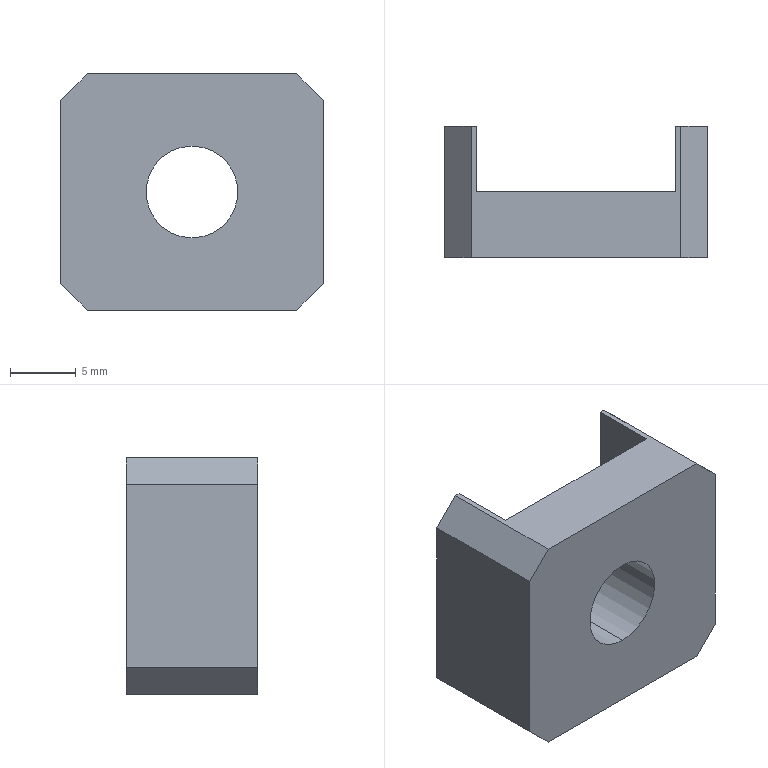Part | STEP file | con chan chot xien | 1 solid | 16 faces | box 20 x 10 x 18 mm | volume 1960 mm3 | plane 14 | cylinder 2 | commonest cylinder face diameters 7 x2
STEP:
#1=CARTESIAN_POINT('',(0.,0.,0.));
#2=DIRECTION('',(0.,0.,1.));
#3=DIRECTION('',(1.,0.,0.));
#4=AXIS2_PLACEMENT_3D('',#1,#2,#3);
#5=CARTESIAN_POINT('',(10.,5.,5.5));
#6=VERTEX_POINT('',#5);
#7=CARTESIAN_POINT('',(10.,0.,5.5));
#8=VERTEX_POINT('',#7);
#9=CARTESIAN_POINT('',(10.,28.705,5.5));
#10=DIRECTION('',(0.,-1.,0.));
#11=VECTOR('',#10,1.);
#12=LINE('',#9,#11);
#13=CARTESIAN_POINT('',(10.,28.705,9.));
#14=DIRECTION('',(0.,-1.,0.));
#15=DIRECTION('',(0.,0.,-1.));
#16=AXIS2_PLACEMENT_3D('',#13,#14,#15);
#17=CYLINDRICAL_SURFACE('',#16,3.5);
#18=CARTESIAN_POINT('',(6.283,0.));
#19=DIRECTION('',(0.,1.));
#20=VECTOR('',#19,1.);
#21=LINE('',#18,#20);
#22=(GEOMETRIC_REPRESENTATION_CONTEXT(2)PARAMETRIC_REPRESENTATION_CONTEXT()REPRESENTATION_CONTEXT('',''));
#23=DEFINITIONAL_REPRESENTATION('',(#21),#22);
#24=PCURVE('',#17,#23);
#25=CARTESIAN_POINT('',(10.,28.705,9.));
#26=DIRECTION('',(0.,-1.,0.));
#27=DIRECTION('',(0.,0.,-1.));
#28=AXIS2_PLACEMENT_3D('',#25,#26,#27);
#29=CYLINDRICAL_SURFACE('',#28,3.5);
#30=CARTESIAN_POINT('',(0.,0.));
#31=DIRECTION('',(0.,1.));
#32=VECTOR('',#31,1.);
#33=LINE('',#30,#32);
#34=(GEOMETRIC_REPRESENTATION_CONTEXT(2)PARAMETRIC_REPRESENTATION_CONTEXT()REPRESENTATION_CONTEXT('',''));
#35=DEFINITIONAL_REPRESENTATION('',(#33),#34);
#36=PCURVE('',#29,#35);
#37=SURFACE_CURVE('',#12,(#24,#36),.PCURVE_S1.);
#38=EDGE_CURVE('',#6,#8,#37,.T.);
#39=ORIENTED_EDGE('',*,*,#38,.T.);
#40=CARTESIAN_POINT('',(10.,0.,12.5));
#41=VERTEX_POINT('',#40);
#42=CARTESIAN_POINT('',(10.,0.,9.));
#43=DIRECTION('',(0.,1.,0.));
#44=DIRECTION('',(0.,0.,-1.));
#45=AXIS2_PLACEMENT_3D('',#42,#43,#44);
#46=CIRCLE('',#45,3.5);
#47=CARTESIAN_POINT('',(6.283,28.705));
#48=DIRECTION('',(-1.,0.));
#49=VECTOR('',#48,1.);
#50=LINE('',#47,#49);
#51=(GEOMETRIC_REPRESENTATION_CONTEXT(2)PARAMETRIC_REPRESENTATION_CONTEXT()REPRESENTATION_CONTEXT('',''));
#52=DEFINITIONAL_REPRESENTATION('',(#50),#51);
#53=PCURVE('',#17,#52);
#54=CARTESIAN_POINT('',(20.,0.,0.));
#55=DIRECTION('',(0.,-1.,0.));
#56=DIRECTION('',(0.,0.,-1.));
#57=AXIS2_PLACEMENT_3D('',#54,#55,#56);
#58=PLANE('',#57);
#59=CARTESIAN_POINT('',(-5.5,-10.));
#60=CARTESIAN_POINT('',(-5.5,-16.062));
#61=CARTESIAN_POINT('',(-10.75,-13.031));
#62=CARTESIAN_POINT('',(-16.,-10.));
#63=CARTESIAN_POINT('',(-10.75,-6.969));
#64=CARTESIAN_POINT('',(-5.5,-3.938));
#65=CARTESIAN_POINT('',(-5.5,-10.));
#66=(BOUNDED_CURVE()B_SPLINE_CURVE(2,(#59,#60,#61,#62,#63,#64,#65),.UNSPECIFIED.,.T.,.F.)B_SPLINE_CURVE_WITH_KNOTS((1,2,2,2,2,1),(-2.094,0.,2.094,4.189,6.283,8.378),.UNSPECIFIED.)CURVE()GEOMETRIC_REPRESENTATION_ITEM()RATIONAL_B_SPLINE_CURVE((1.,0.5,1.,0.5,1.,0.5,1.))REPRESENTATION_ITEM(''));
#67=(GEOMETRIC_REPRESENTATION_CONTEXT(2)PARAMETRIC_REPRESENTATION_CONTEXT()REPRESENTATION_CONTEXT('',''));
#68=DEFINITIONAL_REPRESENTATION('',(#66),#67);
#69=PCURVE('',#58,#68);
#70=SURFACE_CURVE('',#46,(#53,#69),.PCURVE_S1.);
#71=EDGE_CURVE('',#8,#41,#70,.T.);
#72=ORIENTED_EDGE('',*,*,#71,.T.);
#73=CARTESIAN_POINT('',(10.,5.,12.5));
#74=VERTEX_POINT('',#73);
#75=CARTESIAN_POINT('',(10.,28.705,12.5));
#76=DIRECTION('',(0.,-1.,0.));
#77=VECTOR('',#76,1.);
#78=LINE('',#75,#77);
#79=CARTESIAN_POINT('',(3.142,0.));
#80=DIRECTION('',(0.,1.));
#81=VECTOR('',#80,1.);
#82=LINE('',#79,#81);
#83=(GEOMETRIC_REPRESENTATION_CONTEXT(2)PARAMETRIC_REPRESENTATION_CONTEXT()REPRESENTATION_CONTEXT('',''));
#84=DEFINITIONAL_REPRESENTATION('',(#82),#83);
#85=PCURVE('',#17,#84);
#86=CARTESIAN_POINT('',(3.142,0.));
#87=DIRECTION('',(0.,1.));
#88=VECTOR('',#87,1.);
#89=LINE('',#86,#88);
#90=(GEOMETRIC_REPRESENTATION_CONTEXT(2)PARAMETRIC_REPRESENTATION_CONTEXT()REPRESENTATION_CONTEXT('',''));
#91=DEFINITIONAL_REPRESENTATION('',(#89),#90);
#92=PCURVE('',#29,#91);
#93=SURFACE_CURVE('',#78,(#85,#92),.PCURVE_S1.);
#94=EDGE_CURVE('',#74,#41,#93,.T.);
#95=ORIENTED_EDGE('',*,*,#94,.F.);
#96=CARTESIAN_POINT('',(10.,5.,9.));
#97=DIRECTION('',(0.,-1.,0.));
#98=DIRECTION('',(0.,0.,-1.));
#99=AXIS2_PLACEMENT_3D('',#96,#97,#98);
#100=CIRCLE('',#99,3.5);
#101=CARTESIAN_POINT('',(0.,23.705));
#102=DIRECTION('',(1.,0.));
#103=VECTOR('',#102,1.);
#104=LINE('',#101,#103);
#105=(GEOMETRIC_REPRESENTATION_CONTEXT(2)PARAMETRIC_REPRESENTATION_CONTEXT()REPRESENTATION_CONTEXT('',''));
#106=DEFINITIONAL_REPRESENTATION('',(#104),#105);
#107=PCURVE('',#17,#106);
#108=CARTESIAN_POINT('',(2.4,5.,0.));
#109=DIRECTION('',(0.,1.,0.));
#110=DIRECTION('',(0.,0.,1.));
#111=AXIS2_PLACEMENT_3D('',#108,#109,#110);
#112=PLANE('',#111);
#113=CARTESIAN_POINT('',(5.5,7.6));
#114=CARTESIAN_POINT('',(5.5,13.662));
#115=CARTESIAN_POINT('',(10.75,10.631));
#116=CARTESIAN_POINT('',(16.,7.6));
#117=CARTESIAN_POINT('',(10.75,4.569));
#118=CARTESIAN_POINT('',(5.5,1.538));
#119=CARTESIAN_POINT('',(5.5,7.6));
#120=(BOUNDED_CURVE()B_SPLINE_CURVE(2,(#113,#114,#115,#116,#117,#118,#119),.UNSPECIFIED.,.T.,.F.)B_SPLINE_CURVE_WITH_KNOTS((1,2,2,2,2,1),(-2.094,0.,2.094,4.189,6.283,8.378),.UNSPECIFIED.)CURVE()GEOMETRIC_REPRESENTATION_ITEM()RATIONAL_B_SPLINE_CURVE((1.,0.5,1.,0.5,1.,0.5,1.))REPRESENTATION_ITEM(''));
#121=(GEOMETRIC_REPRESENTATION_CONTEXT(2)PARAMETRIC_REPRESENTATION_CONTEXT()REPRESENTATION_CONTEXT('',''));
#122=DEFINITIONAL_REPRESENTATION('',(#120),#121);
#123=PCURVE('',#112,#122);
#124=SURFACE_CURVE('',#100,(#107,#123),.PCURVE_S1.);
#125=EDGE_CURVE('',#74,#6,#124,.T.);
#126=ORIENTED_EDGE('',*,*,#125,.T.);
#127=EDGE_LOOP('',(#39,#72,#95,#126));
#128=FACE_BOUND('',#127,.F.);
#129=ADVANCED_FACE('',(#128),#17,.F.);
#130=ORIENTED_EDGE('',*,*,#71,.T.);
#131=CARTESIAN_POINT('',(10.,0.,9.));
#132=DIRECTION('',(0.,1.,0.));
#133=DIRECTION('',(0.,0.,-1.));
#134=AXIS2_PLACEMENT_3D('',#131,#132,#133);
#135=CIRCLE('',#134,3.5);
#136=CARTESIAN_POINT('',(-5.5,-10.));
#137=CARTESIAN_POINT('',(-5.5,-16.062));
#138=CARTESIAN_POINT('',(-10.75,-13.031));
#139=CARTESIAN_POINT('',(-16.,-10.));
#140=CARTESIAN_POINT('',(-10.75,-6.969));
#141=CARTESIAN_POINT('',(-5.5,-3.938));
#142=CARTESIAN_POINT('',(-5.5,-10.));
#143=(BOUNDED_CURVE()B_SPLINE_CURVE(2,(#136,#137,#138,#139,#140,#141,#142),.UNSPECIFIED.,.T.,.F.)B_SPLINE_CURVE_WITH_KNOTS((1,2,2,2,2,1),(-2.094,0.,2.094,4.189,6.283,8.378),.UNSPECIFIED.)CURVE()GEOMETRIC_REPRESENTATION_ITEM()RATIONAL_B_SPLINE_CURVE((1.,0.5,1.,0.5,1.,0.5,1.))REPRESENTATION_ITEM(''));
#144=(GEOMETRIC_REPRESENTATION_CONTEXT(2)PARAMETRIC_REPRESENTATION_CONTEXT()REPRESENTATION_CONTEXT('',''));
#145=DEFINITIONAL_REPRESENTATION('',(#143),#144);
#146=PCURVE('',#58,#145);
#147=CARTESIAN_POINT('',(6.283,28.705));
#148=DIRECTION('',(-1.,0.));
#149=VECTOR('',#148,1.);
#150=LINE('',#147,#149);
#151=(GEOMETRIC_REPRESENTATION_CONTEXT(2)PARAMETRIC_REPRESENTATION_CONTEXT()REPRESENTATION_CONTEXT('',''));
#152=DEFINITIONAL_REPRESENTATION('',(#150),#151);
#153=PCURVE('',#29,#152);
#154=SURFACE_CURVE('',#135,(#146,#153),.PCURVE_S1.);
#155=EDGE_CURVE('',#41,#8,#154,.T.);
#156=ORIENTED_EDGE('',*,*,#155,.T.);
#157=EDGE_LOOP('',(#130,#156));
#158=FACE_BOUND('',#157,.T.);
#159=CARTESIAN_POINT('',(18.,0.,0.));
#160=VERTEX_POINT('',#159);
#161=CARTESIAN_POINT('',(20.,0.,2.));
#162=VERTEX_POINT('',#161);
#163=CARTESIAN_POINT('',(18.,0.,0.));
#164=DIRECTION('',(0.7071,0.,0.7071));
#165=VECTOR('',#164,1.);
#166=LINE('',#163,#165);
#167=CARTESIAN_POINT('',(0.,-2.));
#168=DIRECTION('',(-0.7071,0.7071));
#169=VECTOR('',#168,1.);
#170=LINE('',#167,#169);
#171=(GEOMETRIC_REPRESENTATION_CONTEXT(2)PARAMETRIC_REPRESENTATION_CONTEXT()REPRESENTATION_CONTEXT('',''));
#172=DEFINITIONAL_REPRESENTATION('',(#170),#171);
#173=PCURVE('',#58,#172);
#174=CARTESIAN_POINT('',(19.,7.136,1.));
#175=DIRECTION('',(0.7071,0.,-0.7071));
#176=DIRECTION('',(-0.7071,0.,-0.7071));
#177=AXIS2_PLACEMENT_3D('',#174,#175,#176);
#178=PLANE('',#177);
#179=CARTESIAN_POINT('',(1.414,-7.136));
#180=DIRECTION('',(-1.,0.));
#181=VECTOR('',#180,1.);
#182=LINE('',#179,#181);
#183=(GEOMETRIC_REPRESENTATION_CONTEXT(2)PARAMETRIC_REPRESENTATION_CONTEXT()REPRESENTATION_CONTEXT('',''));
#184=DEFINITIONAL_REPRESENTATION('',(#182),#183);
#185=PCURVE('',#178,#184);
#186=SURFACE_CURVE('',#166,(#173,#185),.PCURVE_S1.);
#187=EDGE_CURVE('',#160,#162,#186,.T.);
#188=ORIENTED_EDGE('',*,*,#187,.T.);
#189=CARTESIAN_POINT('',(20.,0.,16.));
#190=VERTEX_POINT('',#189);
#191=CARTESIAN_POINT('',(20.,0.,0.));
#192=DIRECTION('',(0.,0.,1.));
#193=VECTOR('',#192,1.);
#194=LINE('',#191,#193);
#195=CARTESIAN_POINT('',(0.,0.));
#196=DIRECTION('',(-1.,0.));
#197=VECTOR('',#196,1.);
#198=LINE('',#195,#197);
#199=(GEOMETRIC_REPRESENTATION_CONTEXT(2)PARAMETRIC_REPRESENTATION_CONTEXT()REPRESENTATION_CONTEXT('',''));
#200=DEFINITIONAL_REPRESENTATION('',(#198),#199);
#201=PCURVE('',#58,#200);
#202=CARTESIAN_POINT('',(20.,10.,0.));
#203=DIRECTION('',(1.,0.,0.));
#204=DIRECTION('',(0.,0.,-1.));
#205=AXIS2_PLACEMENT_3D('',#202,#203,#204);
#206=PLANE('',#205);
#207=CARTESIAN_POINT('',(0.,-10.));
#208=DIRECTION('',(-1.,0.));
#209=VECTOR('',#208,1.);
#210=LINE('',#207,#209);
#211=(GEOMETRIC_REPRESENTATION_CONTEXT(2)PARAMETRIC_REPRESENTATION_CONTEXT()REPRESENTATION_CONTEXT('',''));
#212=DEFINITIONAL_REPRESENTATION('',(#210),#211);
#213=PCURVE('',#206,#212);
#214=SURFACE_CURVE('',#194,(#201,#213),.PCURVE_S1.);
#215=EDGE_CURVE('',#162,#190,#214,.T.);
#216=ORIENTED_EDGE('',*,*,#215,.T.);
#217=CARTESIAN_POINT('',(18.,0.,18.));
#218=VERTEX_POINT('',#217);
#219=CARTESIAN_POINT('',(20.,0.,16.));
#220=DIRECTION('',(-0.7071,0.,0.7071));
#221=VECTOR('',#220,1.);
#222=LINE('',#219,#221);
#223=CARTESIAN_POINT('',(-16.,0.));
#224=DIRECTION('',(-0.7071,-0.7071));
#225=VECTOR('',#224,1.);
#226=LINE('',#223,#225);
#227=(GEOMETRIC_REPRESENTATION_CONTEXT(2)PARAMETRIC_REPRESENTATION_CONTEXT()REPRESENTATION_CONTEXT('',''));
#228=DEFINITIONAL_REPRESENTATION('',(#226),#227);
#229=PCURVE('',#58,#228);
#230=CARTESIAN_POINT('',(19.,7.136,17.));
#231=DIRECTION('',(0.7071,0.,0.7071));
#232=DIRECTION('',(0.7071,0.,-0.7071));
#233=AXIS2_PLACEMENT_3D('',#230,#231,#232);
#234=PLANE('',#233);
#235=CARTESIAN_POINT('',(1.414,-7.136));
#236=DIRECTION('',(-1.,0.));
#237=VECTOR('',#236,1.);
#238=LINE('',#235,#237);
#239=(GEOMETRIC_REPRESENTATION_CONTEXT(2)PARAMETRIC_REPRESENTATION_CONTEXT()REPRESENTATION_CONTEXT('',''));
#240=DEFINITIONAL_REPRESENTATION('',(#238),#239);
#241=PCURVE('',#234,#240);
#242=SURFACE_CURVE('',#222,(#229,#241),.PCURVE_S1.);
#243=EDGE_CURVE('',#190,#218,#242,.T.);
#244=ORIENTED_EDGE('',*,*,#243,.T.);
#245=CARTESIAN_POINT('',(2.,0.,18.));
#246=VERTEX_POINT('',#245);
#247=CARTESIAN_POINT('',(20.,0.,18.));
#248=DIRECTION('',(-1.,0.,0.));
#249=VECTOR('',#248,1.);
#250=LINE('',#247,#249);
#251=CARTESIAN_POINT('',(-18.,0.));
#252=DIRECTION('',(0.,-1.));
#253=VECTOR('',#252,1.);
#254=LINE('',#251,#253);
#255=(GEOMETRIC_REPRESENTATION_CONTEXT(2)PARAMETRIC_REPRESENTATION_CONTEXT()REPRESENTATION_CONTEXT('',''));
#256=DEFINITIONAL_REPRESENTATION('',(#254),#255);
#257=PCURVE('',#58,#256);
#258=CARTESIAN_POINT('',(10.,4.271,18.));
#259=DIRECTION('',(0.,0.,1.));
#260=DIRECTION('',(1.,0.,0.));
#261=AXIS2_PLACEMENT_3D('',#258,#259,#260);
#262=PLANE('',#261);
#263=CARTESIAN_POINT('',(10.,-4.271));
#264=DIRECTION('',(-1.,0.));
#265=VECTOR('',#264,1.);
#266=LINE('',#263,#265);
#267=(GEOMETRIC_REPRESENTATION_CONTEXT(2)PARAMETRIC_REPRESENTATION_CONTEXT()REPRESENTATION_CONTEXT('',''));
#268=DEFINITIONAL_REPRESENTATION('',(#266),#267);
#269=PCURVE('',#262,#268);
#270=SURFACE_CURVE('',#250,(#257,#269),.PCURVE_S1.);
#271=EDGE_CURVE('',#218,#246,#270,.T.);
#272=ORIENTED_EDGE('',*,*,#271,.T.);
#273=CARTESIAN_POINT('',(0.,0.,16.));
#274=VERTEX_POINT('',#273);
#275=CARTESIAN_POINT('',(2.,0.,18.));
#276=DIRECTION('',(-0.7071,0.,-0.7071));
#277=VECTOR('',#276,1.);
#278=LINE('',#275,#277);
#279=CARTESIAN_POINT('',(-18.,-18.));
#280=DIRECTION('',(0.7071,-0.7071));
#281=VECTOR('',#280,1.);
#282=LINE('',#279,#281);
#283=(GEOMETRIC_REPRESENTATION_CONTEXT(2)PARAMETRIC_REPRESENTATION_CONTEXT()REPRESENTATION_CONTEXT('',''));
#284=DEFINITIONAL_REPRESENTATION('',(#282),#283);
#285=PCURVE('',#58,#284);
#286=CARTESIAN_POINT('',(1.,2.136,17.));
#287=DIRECTION('',(-0.7071,0.,0.7071));
#288=DIRECTION('',(0.7071,0.,0.7071));
#289=AXIS2_PLACEMENT_3D('',#286,#287,#288);
#290=PLANE('',#289);
#291=CARTESIAN_POINT('',(1.414,-2.136));
#292=DIRECTION('',(-1.,0.));
#293=VECTOR('',#292,1.);
#294=LINE('',#291,#293);
#295=(GEOMETRIC_REPRESENTATION_CONTEXT(2)PARAMETRIC_REPRESENTATION_CONTEXT()REPRESENTATION_CONTEXT('',''));
#296=DEFINITIONAL_REPRESENTATION('',(#294),#295);
#297=PCURVE('',#290,#296);
#298=SURFACE_CURVE('',#278,(#285,#297),.PCURVE_S1.);
#299=EDGE_CURVE('',#246,#274,#298,.T.);
#300=ORIENTED_EDGE('',*,*,#299,.T.);
#301=CARTESIAN_POINT('',(0.,0.,2.));
#302=VERTEX_POINT('',#301);
#303=CARTESIAN_POINT('',(0.,0.,0.));
#304=DIRECTION('',(0.,0.,-1.));
#305=VECTOR('',#304,1.);
#306=LINE('',#303,#305);
#307=CARTESIAN_POINT('',(0.,-20.));
#308=DIRECTION('',(1.,0.));
#309=VECTOR('',#308,1.);
#310=LINE('',#307,#309);
#311=(GEOMETRIC_REPRESENTATION_CONTEXT(2)PARAMETRIC_REPRESENTATION_CONTEXT()REPRESENTATION_CONTEXT('',''));
#312=DEFINITIONAL_REPRESENTATION('',(#310),#311);
#313=PCURVE('',#58,#312);
#314=CARTESIAN_POINT('',(0.,0.,0.));
#315=DIRECTION('',(-1.,0.,0.));
#316=DIRECTION('',(0.,0.,1.));
#317=AXIS2_PLACEMENT_3D('',#314,#315,#316);
#318=PLANE('',#317);
#319=CARTESIAN_POINT('',(0.,0.));
#320=DIRECTION('',(-1.,0.));
#321=VECTOR('',#320,1.);
#322=LINE('',#319,#321);
#323=(GEOMETRIC_REPRESENTATION_CONTEXT(2)PARAMETRIC_REPRESENTATION_CONTEXT()REPRESENTATION_CONTEXT('',''));
#324=DEFINITIONAL_REPRESENTATION('',(#322),#323);
#325=PCURVE('',#318,#324);
#326=SURFACE_CURVE('',#306,(#313,#325),.PCURVE_S1.);
#327=EDGE_CURVE('',#274,#302,#326,.T.);
#328=ORIENTED_EDGE('',*,*,#327,.T.);
#329=CARTESIAN_POINT('',(2.,0.,0.));
#330=VERTEX_POINT('',#329);
#331=CARTESIAN_POINT('',(0.,0.,2.));
#332=DIRECTION('',(0.7071,0.,-0.7071));
#333=VECTOR('',#332,1.);
#334=LINE('',#331,#333);
#335=CARTESIAN_POINT('',(-2.,-20.));
#336=DIRECTION('',(0.7071,0.7071));
#337=VECTOR('',#336,1.);
#338=LINE('',#335,#337);
#339=(GEOMETRIC_REPRESENTATION_CONTEXT(2)PARAMETRIC_REPRESENTATION_CONTEXT()REPRESENTATION_CONTEXT('',''));
#340=DEFINITIONAL_REPRESENTATION('',(#338),#339);
#341=PCURVE('',#58,#340);
#342=CARTESIAN_POINT('',(1.,2.136,1.));
#343=DIRECTION('',(-0.7071,0.,-0.7071));
#344=DIRECTION('',(-0.7071,0.,0.7071));
#345=AXIS2_PLACEMENT_3D('',#342,#343,#344);
#346=PLANE('',#345);
#347=CARTESIAN_POINT('',(1.414,-2.136));
#348=DIRECTION('',(-1.,0.));
#349=VECTOR('',#348,1.);
#350=LINE('',#347,#349);
#351=(GEOMETRIC_REPRESENTATION_CONTEXT(2)PARAMETRIC_REPRESENTATION_CONTEXT()REPRESENTATION_CONTEXT('',''));
#352=DEFINITIONAL_REPRESENTATION('',(#350),#351);
#353=PCURVE('',#346,#352);
#354=SURFACE_CURVE('',#334,(#341,#353),.PCURVE_S1.);
#355=EDGE_CURVE('',#302,#330,#354,.T.);
#356=ORIENTED_EDGE('',*,*,#355,.T.);
#357=CARTESIAN_POINT('',(20.,0.,0.));
#358=DIRECTION('',(1.,0.,0.));
#359=VECTOR('',#358,1.);
#360=LINE('',#357,#359);
#361=CARTESIAN_POINT('',(0.,0.));
#362=DIRECTION('',(0.,1.));
#363=VECTOR('',#362,1.);
#364=LINE('',#361,#363);
#365=(GEOMETRIC_REPRESENTATION_CONTEXT(2)PARAMETRIC_REPRESENTATION_CONTEXT()REPRESENTATION_CONTEXT('',''));
#366=DEFINITIONAL_REPRESENTATION('',(#364),#365);
#367=PCURVE('',#58,#366);
#368=CARTESIAN_POINT('',(10.,4.271,0.));
#369=DIRECTION('',(0.,0.,1.));
#370=DIRECTION('',(1.,0.,0.));
#371=AXIS2_PLACEMENT_3D('',#368,#369,#370);
#372=PLANE('',#371);
#373=CARTESIAN_POINT('',(10.,-4.271));
#374=DIRECTION('',(1.,0.));
#375=VECTOR('',#374,1.);
#376=LINE('',#373,#375);
#377=(GEOMETRIC_REPRESENTATION_CONTEXT(2)PARAMETRIC_REPRESENTATION_CONTEXT()REPRESENTATION_CONTEXT('',''));
#378=DEFINITIONAL_REPRESENTATION('',(#376),#377);
#379=PCURVE('',#372,#378);
#380=SURFACE_CURVE('',#360,(#367,#379),.PCURVE_S1.);
#381=EDGE_CURVE('',#330,#160,#380,.T.);
#382=ORIENTED_EDGE('',*,*,#381,.T.);
#383=EDGE_LOOP('',(#188,#216,#244,#272,#300,#328,#356,#382));
#384=FACE_BOUND('',#383,.T.);
#385=ADVANCED_FACE('',(#158,#384),#58,.T.);
#386=ORIENTED_EDGE('',*,*,#155,.T.);
#387=ORIENTED_EDGE('',*,*,#38,.F.);
#388=CARTESIAN_POINT('',(10.,5.,9.));
#389=DIRECTION('',(0.,-1.,0.));
#390=DIRECTION('',(0.,0.,-1.));
#391=AXIS2_PLACEMENT_3D('',#388,#389,#390);
#392=CIRCLE('',#391,3.5);
#393=CARTESIAN_POINT('',(0.,23.705));
#394=DIRECTION('',(1.,0.));
#395=VECTOR('',#394,1.);
#396=LINE('',#393,#395);
#397=(GEOMETRIC_REPRESENTATION_CONTEXT(2)PARAMETRIC_REPRESENTATION_CONTEXT()REPRESENTATION_CONTEXT('',''));
#398=DEFINITIONAL_REPRESENTATION('',(#396),#397);
#399=PCURVE('',#29,#398);
#400=CARTESIAN_POINT('',(5.5,7.6));
#401=CARTESIAN_POINT('',(5.5,13.662));
#402=CARTESIAN_POINT('',(10.75,10.631));
#403=CARTESIAN_POINT('',(16.,7.6));
#404=CARTESIAN_POINT('',(10.75,4.569));
#405=CARTESIAN_POINT('',(5.5,1.538));
#406=CARTESIAN_POINT('',(5.5,7.6));
#407=(BOUNDED_CURVE()B_SPLINE_CURVE(2,(#400,#401,#402,#403,#404,#405,#406),.UNSPECIFIED.,.T.,.F.)B_SPLINE_CURVE_WITH_KNOTS((1,2,2,2,2,1),(-2.094,0.,2.094,4.189,6.283,8.378),.UNSPECIFIED.)CURVE()GEOMETRIC_REPRESENTATION_ITEM()RATIONAL_B_SPLINE_CURVE((1.,0.5,1.,0.5,1.,0.5,1.))REPRESENTATION_ITEM(''));
#408=(GEOMETRIC_REPRESENTATION_CONTEXT(2)PARAMETRIC_REPRESENTATION_CONTEXT()REPRESENTATION_CONTEXT('',''));
#409=DEFINITIONAL_REPRESENTATION('',(#407),#408);
#410=PCURVE('',#112,#409);
#411=SURFACE_CURVE('',#392,(#399,#410),.PCURVE_S1.);
#412=EDGE_CURVE('',#6,#74,#411,.T.);
#413=ORIENTED_EDGE('',*,*,#412,.T.);
#414=ORIENTED_EDGE('',*,*,#94,.T.);
#415=EDGE_LOOP('',(#386,#387,#413,#414));
#416=FACE_BOUND('',#415,.F.);
#417=ADVANCED_FACE('',(#416),#29,.F.);
#418=CARTESIAN_POINT('',(20.,10.,2.));
#419=VERTEX_POINT('',#418);
#420=CARTESIAN_POINT('',(20.,10.,2.));
#421=DIRECTION('',(0.,1.,0.));
#422=VECTOR('',#421,1.);
#423=LINE('',#420,#422);
#424=CARTESIAN_POINT('',(-2.,0.));
#425=DIRECTION('',(0.,1.));
#426=VECTOR('',#425,1.);
#427=LINE('',#424,#426);
#428=(GEOMETRIC_REPRESENTATION_CONTEXT(2)PARAMETRIC_REPRESENTATION_CONTEXT()REPRESENTATION_CONTEXT('',''));
#429=DEFINITIONAL_REPRESENTATION('',(#427),#428);
#430=PCURVE('',#206,#429);
#431=CARTESIAN_POINT('',(-1.414,2.864));
#432=DIRECTION('',(0.,1.));
#433=VECTOR('',#432,1.);
#434=LINE('',#431,#433);
#435=(GEOMETRIC_REPRESENTATION_CONTEXT(2)PARAMETRIC_REPRESENTATION_CONTEXT()REPRESENTATION_CONTEXT('',''));
#436=DEFINITIONAL_REPRESENTATION('',(#434),#435);
#437=PCURVE('',#178,#436);
#438=SURFACE_CURVE('',#423,(#430,#437),.PCURVE_S1.);
#439=EDGE_CURVE('',#162,#419,#438,.T.);
#440=ORIENTED_EDGE('',*,*,#439,.T.);
#441=CARTESIAN_POINT('',(20.,10.,16.));
#442=VERTEX_POINT('',#441);
#443=CARTESIAN_POINT('',(20.,10.,0.));
#444=DIRECTION('',(0.,0.,1.));
#445=VECTOR('',#444,1.);
#446=LINE('',#443,#445);
#447=CARTESIAN_POINT('',(0.,0.));
#448=DIRECTION('',(-1.,0.));
#449=VECTOR('',#448,1.);
#450=LINE('',#447,#449);
#451=(GEOMETRIC_REPRESENTATION_CONTEXT(2)PARAMETRIC_REPRESENTATION_CONTEXT()REPRESENTATION_CONTEXT('',''));
#452=DEFINITIONAL_REPRESENTATION('',(#450),#451);
#453=PCURVE('',#206,#452);
#454=CARTESIAN_POINT('',(17.6,10.,0.));
#455=DIRECTION('',(0.,1.,0.));
#456=DIRECTION('',(0.,0.,1.));
#457=AXIS2_PLACEMENT_3D('',#454,#455,#456);
#458=PLANE('',#457);
#459=CARTESIAN_POINT('',(0.,2.4));
#460=DIRECTION('',(1.,0.));
#461=VECTOR('',#460,1.);
#462=LINE('',#459,#461);
#463=(GEOMETRIC_REPRESENTATION_CONTEXT(2)PARAMETRIC_REPRESENTATION_CONTEXT()REPRESENTATION_CONTEXT('',''));
#464=DEFINITIONAL_REPRESENTATION('',(#462),#463);
#465=PCURVE('',#458,#464);
#466=SURFACE_CURVE('',#446,(#453,#465),.PCURVE_S1.);
#467=EDGE_CURVE('',#419,#442,#466,.T.);
#468=ORIENTED_EDGE('',*,*,#467,.T.);
#469=CARTESIAN_POINT('',(20.,10.,16.));
#470=DIRECTION('',(0.,-1.,0.));
#471=VECTOR('',#470,1.);
#472=LINE('',#469,#471);
#473=CARTESIAN_POINT('',(-16.,0.));
#474=DIRECTION('',(0.,-1.));
#475=VECTOR('',#474,1.);
#476=LINE('',#473,#475);
#477=(GEOMETRIC_REPRESENTATION_CONTEXT(2)PARAMETRIC_REPRESENTATION_CONTEXT()REPRESENTATION_CONTEXT('',''));
#478=DEFINITIONAL_REPRESENTATION('',(#476),#477);
#479=PCURVE('',#206,#478);
#480=CARTESIAN_POINT('',(1.414,2.864));
#481=DIRECTION('',(0.,-1.));
#482=VECTOR('',#481,1.);
#483=LINE('',#480,#482);
#484=(GEOMETRIC_REPRESENTATION_CONTEXT(2)PARAMETRIC_REPRESENTATION_CONTEXT()REPRESENTATION_CONTEXT('',''));
#485=DEFINITIONAL_REPRESENTATION('',(#483),#484);
#486=PCURVE('',#234,#485);
#487=SURFACE_CURVE('',#472,(#479,#486),.PCURVE_S1.);
#488=EDGE_CURVE('',#442,#190,#487,.T.);
#489=ORIENTED_EDGE('',*,*,#488,.T.);
#490=ORIENTED_EDGE('',*,*,#215,.F.);
#491=EDGE_LOOP('',(#440,#468,#489,#490));
#492=FACE_BOUND('',#491,.T.);
#493=ADVANCED_FACE('',(#492),#206,.T.);
#494=ORIENTED_EDGE('',*,*,#187,.F.);
#495=CARTESIAN_POINT('',(18.,10.,0.));
#496=VERTEX_POINT('',#495);
#497=CARTESIAN_POINT('',(18.,7.136,0.));
#498=DIRECTION('',(0.,1.,0.));
#499=VECTOR('',#498,1.);
#500=LINE('',#497,#499);
#501=CARTESIAN_POINT('',(1.414,0.));
#502=DIRECTION('',(0.,1.));
#503=VECTOR('',#502,1.);
#504=LINE('',#501,#503);
#505=(GEOMETRIC_REPRESENTATION_CONTEXT(2)PARAMETRIC_REPRESENTATION_CONTEXT()REPRESENTATION_CONTEXT('',''));
#506=DEFINITIONAL_REPRESENTATION('',(#504),#505);
#507=PCURVE('',#178,#506);
#508=CARTESIAN_POINT('',(8.,2.864));
#509=DIRECTION('',(0.,1.));
#510=VECTOR('',#509,1.);
#511=LINE('',#508,#510);
#512=(GEOMETRIC_REPRESENTATION_CONTEXT(2)PARAMETRIC_REPRESENTATION_CONTEXT()REPRESENTATION_CONTEXT('',''));
#513=DEFINITIONAL_REPRESENTATION('',(#511),#512);
#514=PCURVE('',#372,#513);
#515=SURFACE_CURVE('',#500,(#507,#514),.PCURVE_S1.);
#516=EDGE_CURVE('',#160,#496,#515,.T.);
#517=ORIENTED_EDGE('',*,*,#516,.T.);
#518=CARTESIAN_POINT('',(19.,10.,1.));
#519=DIRECTION('',(0.7071,0.,0.7071));
#520=VECTOR('',#519,1.);
#521=LINE('',#518,#520);
#522=CARTESIAN_POINT('',(0.,2.864));
#523=DIRECTION('',(-1.,0.));
#524=VECTOR('',#523,1.);
#525=LINE('',#522,#524);
#526=(GEOMETRIC_REPRESENTATION_CONTEXT(2)PARAMETRIC_REPRESENTATION_CONTEXT()REPRESENTATION_CONTEXT('',''));
#527=DEFINITIONAL_REPRESENTATION('',(#525),#526);
#528=PCURVE('',#178,#527);
#529=CARTESIAN_POINT('',(1.,1.4));
#530=DIRECTION('',(0.7071,0.7071));
#531=VECTOR('',#530,1.);
#532=LINE('',#529,#531);
#533=(GEOMETRIC_REPRESENTATION_CONTEXT(2)PARAMETRIC_REPRESENTATION_CONTEXT()REPRESENTATION_CONTEXT('',''));
#534=DEFINITIONAL_REPRESENTATION('',(#532),#533);
#535=PCURVE('',#458,#534);
#536=SURFACE_CURVE('',#521,(#528,#535),.PCURVE_S1.);
#537=EDGE_CURVE('',#496,#419,#536,.T.);
#538=ORIENTED_EDGE('',*,*,#537,.T.);
#539=ORIENTED_EDGE('',*,*,#439,.F.);
#540=EDGE_LOOP('',(#494,#517,#538,#539));
#541=FACE_BOUND('',#540,.T.);
#542=ADVANCED_FACE('',(#541),#178,.T.);
#543=ORIENTED_EDGE('',*,*,#381,.F.);
#544=CARTESIAN_POINT('',(2.,10.,0.));
#545=VERTEX_POINT('',#544);
#546=CARTESIAN_POINT('',(2.,4.271,0.));
#547=DIRECTION('',(0.,-1.,0.));
#548=VECTOR('',#547,1.);
#549=LINE('',#546,#548);
#550=CARTESIAN_POINT('',(-8.,0.));
#551=DIRECTION('',(0.,-1.));
#552=VECTOR('',#551,1.);
#553=LINE('',#550,#552);
#554=(GEOMETRIC_REPRESENTATION_CONTEXT(2)PARAMETRIC_REPRESENTATION_CONTEXT()REPRESENTATION_CONTEXT('',''));
#555=DEFINITIONAL_REPRESENTATION('',(#553),#554);
#556=PCURVE('',#372,#555);
#557=CARTESIAN_POINT('',(-1.414,2.136));
#558=DIRECTION('',(0.,-1.));
#559=VECTOR('',#558,1.);
#560=LINE('',#557,#559);
#561=(GEOMETRIC_REPRESENTATION_CONTEXT(2)PARAMETRIC_REPRESENTATION_CONTEXT()REPRESENTATION_CONTEXT('',''));
#562=DEFINITIONAL_REPRESENTATION('',(#560),#561);
#563=PCURVE('',#346,#562);
#564=SURFACE_CURVE('',#549,(#556,#563),.PCURVE_S1.);
#565=EDGE_CURVE('',#545,#330,#564,.T.);
#566=ORIENTED_EDGE('',*,*,#565,.F.);
#567=CARTESIAN_POINT('',(2.4,10.,0.));
#568=VERTEX_POINT('',#567);
#569=CARTESIAN_POINT('',(0.,10.,0.));
#570=DIRECTION('',(-1.,0.,0.));
#571=VECTOR('',#570,1.);
#572=LINE('',#569,#571);
#573=CARTESIAN_POINT('',(-10.,5.729));
#574=DIRECTION('',(-1.,0.));
#575=VECTOR('',#574,1.);
#576=LINE('',#573,#575);
#577=(GEOMETRIC_REPRESENTATION_CONTEXT(2)PARAMETRIC_REPRESENTATION_CONTEXT()REPRESENTATION_CONTEXT('',''));
#578=DEFINITIONAL_REPRESENTATION('',(#576),#577);
#579=PCURVE('',#372,#578);
#580=CARTESIAN_POINT('',(0.,10.,0.));
#581=DIRECTION('',(0.,1.,0.));
#582=DIRECTION('',(0.,0.,1.));
#583=AXIS2_PLACEMENT_3D('',#580,#581,#582);
#584=PLANE('',#583);
#585=CARTESIAN_POINT('',(0.,0.));
#586=DIRECTION('',(0.,-1.));
#587=VECTOR('',#586,1.);
#588=LINE('',#585,#587);
#589=(GEOMETRIC_REPRESENTATION_CONTEXT(2)PARAMETRIC_REPRESENTATION_CONTEXT()REPRESENTATION_CONTEXT('',''));
#590=DEFINITIONAL_REPRESENTATION('',(#588),#589);
#591=PCURVE('',#584,#590);
#592=SURFACE_CURVE('',#572,(#579,#591),.PCURVE_S1.);
#593=EDGE_CURVE('',#568,#545,#592,.T.);
#594=ORIENTED_EDGE('',*,*,#593,.F.);
#595=CARTESIAN_POINT('',(2.4,5.,0.));
#596=VERTEX_POINT('',#595);
#597=CARTESIAN_POINT('',(2.4,4.271,0.));
#598=DIRECTION('',(0.,1.,0.));
#599=VECTOR('',#598,1.);
#600=LINE('',#597,#599);
#601=CARTESIAN_POINT('',(-7.6,0.));
#602=DIRECTION('',(0.,1.));
#603=VECTOR('',#602,1.);
#604=LINE('',#601,#603);
#605=(GEOMETRIC_REPRESENTATION_CONTEXT(2)PARAMETRIC_REPRESENTATION_CONTEXT()REPRESENTATION_CONTEXT('',''));
#606=DEFINITIONAL_REPRESENTATION('',(#604),#605);
#607=PCURVE('',#372,#606);
#608=CARTESIAN_POINT('',(2.4,10.,0.));
#609=DIRECTION('',(1.,0.,0.));
#610=DIRECTION('',(0.,0.,-1.));
#611=AXIS2_PLACEMENT_3D('',#608,#609,#610);
#612=PLANE('',#611);
#613=CARTESIAN_POINT('',(0.,-5.729));
#614=DIRECTION('',(0.,1.));
#615=VECTOR('',#614,1.);
#616=LINE('',#613,#615);
#617=(GEOMETRIC_REPRESENTATION_CONTEXT(2)PARAMETRIC_REPRESENTATION_CONTEXT()REPRESENTATION_CONTEXT('',''));
#618=DEFINITIONAL_REPRESENTATION('',(#616),#617);
#619=PCURVE('',#612,#618);
#620=SURFACE_CURVE('',#600,(#607,#619),.PCURVE_S1.);
#621=EDGE_CURVE('',#596,#568,#620,.T.);
#622=ORIENTED_EDGE('',*,*,#621,.F.);
#623=CARTESIAN_POINT('',(17.6,5.,0.));
#624=VERTEX_POINT('',#623);
#625=CARTESIAN_POINT('',(10.,5.,0.));
#626=DIRECTION('',(-1.,0.,0.));
#627=VECTOR('',#626,1.);
#628=LINE('',#625,#627);
#629=CARTESIAN_POINT('',(0.,0.7286));
#630=DIRECTION('',(-1.,0.));
#631=VECTOR('',#630,1.);
#632=LINE('',#629,#631);
#633=(GEOMETRIC_REPRESENTATION_CONTEXT(2)PARAMETRIC_REPRESENTATION_CONTEXT()REPRESENTATION_CONTEXT('',''));
#634=DEFINITIONAL_REPRESENTATION('',(#632),#633);
#635=PCURVE('',#372,#634);
#636=CARTESIAN_POINT('',(0.,7.6));
#637=DIRECTION('',(0.,-1.));
#638=VECTOR('',#637,1.);
#639=LINE('',#636,#638);
#640=(GEOMETRIC_REPRESENTATION_CONTEXT(2)PARAMETRIC_REPRESENTATION_CONTEXT()REPRESENTATION_CONTEXT('',''));
#641=DEFINITIONAL_REPRESENTATION('',(#639),#640);
#642=PCURVE('',#112,#641);
#643=SURFACE_CURVE('',#628,(#635,#642),.PCURVE_S1.);
#644=EDGE_CURVE('',#624,#596,#643,.T.);
#645=ORIENTED_EDGE('',*,*,#644,.F.);
#646=CARTESIAN_POINT('',(17.6,10.,0.));
#647=VERTEX_POINT('',#646);
#648=CARTESIAN_POINT('',(17.6,4.271,0.));
#649=DIRECTION('',(0.,-1.,0.));
#650=VECTOR('',#649,1.);
#651=LINE('',#648,#650);
#652=CARTESIAN_POINT('',(7.6,0.));
#653=DIRECTION('',(0.,-1.));
#654=VECTOR('',#653,1.);
#655=LINE('',#652,#654);
#656=(GEOMETRIC_REPRESENTATION_CONTEXT(2)PARAMETRIC_REPRESENTATION_CONTEXT()REPRESENTATION_CONTEXT('',''));
#657=DEFINITIONAL_REPRESENTATION('',(#655),#656);
#658=PCURVE('',#372,#657);
#659=CARTESIAN_POINT('',(17.6,5.,0.));
#660=DIRECTION('',(-1.,0.,0.));
#661=DIRECTION('',(0.,0.,1.));
#662=AXIS2_PLACEMENT_3D('',#659,#660,#661);
#663=PLANE('',#662);
#664=CARTESIAN_POINT('',(0.,-0.7286));
#665=DIRECTION('',(0.,-1.));
#666=VECTOR('',#665,1.);
#667=LINE('',#664,#666);
#668=(GEOMETRIC_REPRESENTATION_CONTEXT(2)PARAMETRIC_REPRESENTATION_CONTEXT()REPRESENTATION_CONTEXT('',''));
#669=DEFINITIONAL_REPRESENTATION('',(#667),#668);
#670=PCURVE('',#663,#669);
#671=SURFACE_CURVE('',#651,(#658,#670),.PCURVE_S1.);
#672=EDGE_CURVE('',#647,#624,#671,.T.);
#673=ORIENTED_EDGE('',*,*,#672,.F.);
#674=CARTESIAN_POINT('',(10.,10.,0.));
#675=DIRECTION('',(-1.,0.,0.));
#676=VECTOR('',#675,1.);
#677=LINE('',#674,#676);
#678=CARTESIAN_POINT('',(0.,5.729));
#679=DIRECTION('',(-1.,0.));
#680=VECTOR('',#679,1.);
#681=LINE('',#678,#680);
#682=(GEOMETRIC_REPRESENTATION_CONTEXT(2)PARAMETRIC_REPRESENTATION_CONTEXT()REPRESENTATION_CONTEXT('',''));
#683=DEFINITIONAL_REPRESENTATION('',(#681),#682);
#684=PCURVE('',#372,#683);
#685=CARTESIAN_POINT('',(0.,-7.6));
#686=DIRECTION('',(0.,-1.));
#687=VECTOR('',#686,1.);
#688=LINE('',#685,#687);
#689=(GEOMETRIC_REPRESENTATION_CONTEXT(2)PARAMETRIC_REPRESENTATION_CONTEXT()REPRESENTATION_CONTEXT('',''));
#690=DEFINITIONAL_REPRESENTATION('',(#688),#689);
#691=PCURVE('',#458,#690);
#692=SURFACE_CURVE('',#677,(#684,#691),.PCURVE_S1.);
#693=EDGE_CURVE('',#496,#647,#692,.T.);
#694=ORIENTED_EDGE('',*,*,#693,.F.);
#695=ORIENTED_EDGE('',*,*,#516,.F.);
#696=EDGE_LOOP('',(#543,#566,#594,#622,#645,#673,#694,#695));
#697=FACE_BOUND('',#696,.T.);
#698=ADVANCED_FACE('',(#697),#372,.F.);
#699=CARTESIAN_POINT('',(0.,10.,2.));
#700=VERTEX_POINT('',#699);
#701=CARTESIAN_POINT('',(1.,10.,1.));
#702=DIRECTION('',(0.7071,0.,-0.7071));
#703=VECTOR('',#702,1.);
#704=LINE('',#701,#703);
#705=CARTESIAN_POINT('',(0.,7.864));
#706=DIRECTION('',(-1.,0.));
#707=VECTOR('',#706,1.);
#708=LINE('',#705,#707);
#709=(GEOMETRIC_REPRESENTATION_CONTEXT(2)PARAMETRIC_REPRESENTATION_CONTEXT()REPRESENTATION_CONTEXT('',''));
#710=DEFINITIONAL_REPRESENTATION('',(#708),#709);
#711=PCURVE('',#346,#710);
#712=CARTESIAN_POINT('',(1.,1.));
#713=DIRECTION('',(-0.7071,0.7071));
#714=VECTOR('',#713,1.);
#715=LINE('',#712,#714);
#716=(GEOMETRIC_REPRESENTATION_CONTEXT(2)PARAMETRIC_REPRESENTATION_CONTEXT()REPRESENTATION_CONTEXT('',''));
#717=DEFINITIONAL_REPRESENTATION('',(#715),#716);
#718=PCURVE('',#584,#717);
#719=SURFACE_CURVE('',#704,(#711,#718),.PCURVE_S1.);
#720=EDGE_CURVE('',#700,#545,#719,.T.);
#721=ORIENTED_EDGE('',*,*,#720,.T.);
#722=ORIENTED_EDGE('',*,*,#565,.T.);
#723=ORIENTED_EDGE('',*,*,#355,.F.);
#724=CARTESIAN_POINT('',(0.,2.136,2.));
#725=DIRECTION('',(0.,1.,0.));
#726=VECTOR('',#725,1.);
#727=LINE('',#724,#726);
#728=CARTESIAN_POINT('',(1.414,0.));
#729=DIRECTION('',(0.,1.));
#730=VECTOR('',#729,1.);
#731=LINE('',#728,#730);
#732=(GEOMETRIC_REPRESENTATION_CONTEXT(2)PARAMETRIC_REPRESENTATION_CONTEXT()REPRESENTATION_CONTEXT('',''));
#733=DEFINITIONAL_REPRESENTATION('',(#731),#732);
#734=PCURVE('',#346,#733);
#735=CARTESIAN_POINT('',(2.,2.136));
#736=DIRECTION('',(0.,1.));
#737=VECTOR('',#736,1.);
#738=LINE('',#735,#737);
#739=(GEOMETRIC_REPRESENTATION_CONTEXT(2)PARAMETRIC_REPRESENTATION_CONTEXT()REPRESENTATION_CONTEXT('',''));
#740=DEFINITIONAL_REPRESENTATION('',(#738),#739);
#741=PCURVE('',#318,#740);
#742=SURFACE_CURVE('',#727,(#734,#741),.PCURVE_S1.);
#743=EDGE_CURVE('',#302,#700,#742,.T.);
#744=ORIENTED_EDGE('',*,*,#743,.T.);
#745=EDGE_LOOP('',(#721,#722,#723,#744));
#746=FACE_BOUND('',#745,.T.);
#747=ADVANCED_FACE('',(#746),#346,.T.);
#748=CARTESIAN_POINT('',(0.,10.,16.));
#749=VERTEX_POINT('',#748);
#750=CARTESIAN_POINT('',(0.,0.,16.));
#751=DIRECTION('',(0.,1.,0.));
#752=VECTOR('',#751,1.);
#753=LINE('',#750,#752);
#754=CARTESIAN_POINT('',(16.,0.));
#755=DIRECTION('',(0.,1.));
#756=VECTOR('',#755,1.);
#757=LINE('',#754,#756);
#758=(GEOMETRIC_REPRESENTATION_CONTEXT(2)PARAMETRIC_REPRESENTATION_CONTEXT()REPRESENTATION_CONTEXT('',''));
#759=DEFINITIONAL_REPRESENTATION('',(#757),#758);
#760=PCURVE('',#318,#759);
#761=CARTESIAN_POINT('',(-1.414,-2.136));
#762=DIRECTION('',(0.,1.));
#763=VECTOR('',#762,1.);
#764=LINE('',#761,#763);
#765=(GEOMETRIC_REPRESENTATION_CONTEXT(2)PARAMETRIC_REPRESENTATION_CONTEXT()REPRESENTATION_CONTEXT('',''));
#766=DEFINITIONAL_REPRESENTATION('',(#764),#765);
#767=PCURVE('',#290,#766);
#768=SURFACE_CURVE('',#753,(#760,#767),.PCURVE_S1.);
#769=EDGE_CURVE('',#274,#749,#768,.T.);
#770=ORIENTED_EDGE('',*,*,#769,.T.);
#771=CARTESIAN_POINT('',(0.,10.,0.));
#772=DIRECTION('',(0.,0.,-1.));
#773=VECTOR('',#772,1.);
#774=LINE('',#771,#773);
#775=CARTESIAN_POINT('',(0.,10.));
#776=DIRECTION('',(-1.,0.));
#777=VECTOR('',#776,1.);
#778=LINE('',#775,#777);
#779=(GEOMETRIC_REPRESENTATION_CONTEXT(2)PARAMETRIC_REPRESENTATION_CONTEXT()REPRESENTATION_CONTEXT('',''));
#780=DEFINITIONAL_REPRESENTATION('',(#778),#779);
#781=PCURVE('',#318,#780);
#782=CARTESIAN_POINT('',(0.,0.));
#783=DIRECTION('',(-1.,0.));
#784=VECTOR('',#783,1.);
#785=LINE('',#782,#784);
#786=(GEOMETRIC_REPRESENTATION_CONTEXT(2)PARAMETRIC_REPRESENTATION_CONTEXT()REPRESENTATION_CONTEXT('',''));
#787=DEFINITIONAL_REPRESENTATION('',(#785),#786);
#788=PCURVE('',#584,#787);
#789=SURFACE_CURVE('',#774,(#781,#788),.PCURVE_S1.);
#790=EDGE_CURVE('',#749,#700,#789,.T.);
#791=ORIENTED_EDGE('',*,*,#790,.T.);
#792=ORIENTED_EDGE('',*,*,#743,.F.);
#793=ORIENTED_EDGE('',*,*,#327,.F.);
#794=EDGE_LOOP('',(#770,#791,#792,#793));
#795=FACE_BOUND('',#794,.T.);
#796=ADVANCED_FACE('',(#795),#318,.T.);
#797=ORIENTED_EDGE('',*,*,#299,.F.);
#798=CARTESIAN_POINT('',(2.,10.,18.));
#799=VERTEX_POINT('',#798);
#800=CARTESIAN_POINT('',(2.,2.136,18.));
#801=DIRECTION('',(0.,1.,0.));
#802=VECTOR('',#801,1.);
#803=LINE('',#800,#802);
#804=CARTESIAN_POINT('',(1.414,0.));
#805=DIRECTION('',(0.,1.));
#806=VECTOR('',#805,1.);
#807=LINE('',#804,#806);
#808=(GEOMETRIC_REPRESENTATION_CONTEXT(2)PARAMETRIC_REPRESENTATION_CONTEXT()REPRESENTATION_CONTEXT('',''));
#809=DEFINITIONAL_REPRESENTATION('',(#807),#808);
#810=PCURVE('',#290,#809);
#811=CARTESIAN_POINT('',(-8.,-2.136));
#812=DIRECTION('',(0.,1.));
#813=VECTOR('',#812,1.);
#814=LINE('',#811,#813);
#815=(GEOMETRIC_REPRESENTATION_CONTEXT(2)PARAMETRIC_REPRESENTATION_CONTEXT()REPRESENTATION_CONTEXT('',''));
#816=DEFINITIONAL_REPRESENTATION('',(#814),#815);
#817=PCURVE('',#262,#816);
#818=SURFACE_CURVE('',#803,(#810,#817),.PCURVE_S1.);
#819=EDGE_CURVE('',#246,#799,#818,.T.);
#820=ORIENTED_EDGE('',*,*,#819,.T.);
#821=CARTESIAN_POINT('',(1.,10.,17.));
#822=DIRECTION('',(-0.7071,0.,-0.7071));
#823=VECTOR('',#822,1.);
#824=LINE('',#821,#823);
#825=CARTESIAN_POINT('',(0.,7.864));
#826=DIRECTION('',(-1.,0.));
#827=VECTOR('',#826,1.);
#828=LINE('',#825,#827);
#829=(GEOMETRIC_REPRESENTATION_CONTEXT(2)PARAMETRIC_REPRESENTATION_CONTEXT()REPRESENTATION_CONTEXT('',''));
#830=DEFINITIONAL_REPRESENTATION('',(#828),#829);
#831=PCURVE('',#290,#830);
#832=CARTESIAN_POINT('',(17.,1.));
#833=DIRECTION('',(-0.7071,-0.7071));
#834=VECTOR('',#833,1.);
#835=LINE('',#832,#834);
#836=(GEOMETRIC_REPRESENTATION_CONTEXT(2)PARAMETRIC_REPRESENTATION_CONTEXT()REPRESENTATION_CONTEXT('',''));
#837=DEFINITIONAL_REPRESENTATION('',(#835),#836);
#838=PCURVE('',#584,#837);
#839=SURFACE_CURVE('',#824,(#831,#838),.PCURVE_S1.);
#840=EDGE_CURVE('',#799,#749,#839,.T.);
#841=ORIENTED_EDGE('',*,*,#840,.T.);
#842=ORIENTED_EDGE('',*,*,#769,.F.);
#843=EDGE_LOOP('',(#797,#820,#841,#842));
#844=FACE_BOUND('',#843,.T.);
#845=ADVANCED_FACE('',(#844),#290,.T.);
#846=ORIENTED_EDGE('',*,*,#819,.F.);
#847=ORIENTED_EDGE('',*,*,#271,.F.);
#848=CARTESIAN_POINT('',(18.,10.,18.));
#849=VERTEX_POINT('',#848);
#850=CARTESIAN_POINT('',(18.,4.271,18.));
#851=DIRECTION('',(0.,1.,0.));
#852=VECTOR('',#851,1.);
#853=LINE('',#850,#852);
#854=CARTESIAN_POINT('',(8.,0.));
#855=DIRECTION('',(0.,1.));
#856=VECTOR('',#855,1.);
#857=LINE('',#854,#856);
#858=(GEOMETRIC_REPRESENTATION_CONTEXT(2)PARAMETRIC_REPRESENTATION_CONTEXT()REPRESENTATION_CONTEXT('',''));
#859=DEFINITIONAL_REPRESENTATION('',(#857),#858);
#860=PCURVE('',#262,#859);
#861=CARTESIAN_POINT('',(-1.414,-2.864));
#862=DIRECTION('',(0.,1.));
#863=VECTOR('',#862,1.);
#864=LINE('',#861,#863);
#865=(GEOMETRIC_REPRESENTATION_CONTEXT(2)PARAMETRIC_REPRESENTATION_CONTEXT()REPRESENTATION_CONTEXT('',''));
#866=DEFINITIONAL_REPRESENTATION('',(#864),#865);
#867=PCURVE('',#234,#866);
#868=SURFACE_CURVE('',#853,(#860,#867),.PCURVE_S1.);
#869=EDGE_CURVE('',#218,#849,#868,.T.);
#870=ORIENTED_EDGE('',*,*,#869,.T.);
#871=CARTESIAN_POINT('',(17.6,10.,18.));
#872=VERTEX_POINT('',#871);
#873=CARTESIAN_POINT('',(10.,10.,18.));
#874=DIRECTION('',(-1.,0.,0.));
#875=VECTOR('',#874,1.);
#876=LINE('',#873,#875);
#877=CARTESIAN_POINT('',(0.,5.729));
#878=DIRECTION('',(-1.,0.));
#879=VECTOR('',#878,1.);
#880=LINE('',#877,#879);
#881=(GEOMETRIC_REPRESENTATION_CONTEXT(2)PARAMETRIC_REPRESENTATION_CONTEXT()REPRESENTATION_CONTEXT('',''));
#882=DEFINITIONAL_REPRESENTATION('',(#880),#881);
#883=PCURVE('',#262,#882);
#884=CARTESIAN_POINT('',(18.,-7.6));
#885=DIRECTION('',(0.,-1.));
#886=VECTOR('',#885,1.);
#887=LINE('',#884,#886);
#888=(GEOMETRIC_REPRESENTATION_CONTEXT(2)PARAMETRIC_REPRESENTATION_CONTEXT()REPRESENTATION_CONTEXT('',''));
#889=DEFINITIONAL_REPRESENTATION('',(#887),#888);
#890=PCURVE('',#458,#889);
#891=SURFACE_CURVE('',#876,(#883,#890),.PCURVE_S1.);
#892=EDGE_CURVE('',#849,#872,#891,.T.);
#893=ORIENTED_EDGE('',*,*,#892,.T.);
#894=CARTESIAN_POINT('',(17.6,5.,18.));
#895=VERTEX_POINT('',#894);
#896=CARTESIAN_POINT('',(17.6,4.271,18.));
#897=DIRECTION('',(0.,-1.,0.));
#898=VECTOR('',#897,1.);
#899=LINE('',#896,#898);
#900=CARTESIAN_POINT('',(7.6,0.));
#901=DIRECTION('',(0.,-1.));
#902=VECTOR('',#901,1.);
#903=LINE('',#900,#902);
#904=(GEOMETRIC_REPRESENTATION_CONTEXT(2)PARAMETRIC_REPRESENTATION_CONTEXT()REPRESENTATION_CONTEXT('',''));
#905=DEFINITIONAL_REPRESENTATION('',(#903),#904);
#906=PCURVE('',#262,#905);
#907=CARTESIAN_POINT('',(18.,-0.7286));
#908=DIRECTION('',(0.,-1.));
#909=VECTOR('',#908,1.);
#910=LINE('',#907,#909);
#911=(GEOMETRIC_REPRESENTATION_CONTEXT(2)PARAMETRIC_REPRESENTATION_CONTEXT()REPRESENTATION_CONTEXT('',''));
#912=DEFINITIONAL_REPRESENTATION('',(#910),#911);
#913=PCURVE('',#663,#912);
#914=SURFACE_CURVE('',#899,(#906,#913),.PCURVE_S1.);
#915=EDGE_CURVE('',#872,#895,#914,.T.);
#916=ORIENTED_EDGE('',*,*,#915,.T.);
#917=CARTESIAN_POINT('',(2.4,5.,18.));
#918=VERTEX_POINT('',#917);
#919=CARTESIAN_POINT('',(10.,5.,18.));
#920=DIRECTION('',(-1.,0.,0.));
#921=VECTOR('',#920,1.);
#922=LINE('',#919,#921);
#923=CARTESIAN_POINT('',(0.,0.7286));
#924=DIRECTION('',(-1.,0.));
#925=VECTOR('',#924,1.);
#926=LINE('',#923,#925);
#927=(GEOMETRIC_REPRESENTATION_CONTEXT(2)PARAMETRIC_REPRESENTATION_CONTEXT()REPRESENTATION_CONTEXT('',''));
#928=DEFINITIONAL_REPRESENTATION('',(#926),#927);
#929=PCURVE('',#262,#928);
#930=CARTESIAN_POINT('',(18.,7.6));
#931=DIRECTION('',(0.,-1.));
#932=VECTOR('',#931,1.);
#933=LINE('',#930,#932);
#934=(GEOMETRIC_REPRESENTATION_CONTEXT(2)PARAMETRIC_REPRESENTATION_CONTEXT()REPRESENTATION_CONTEXT('',''));
#935=DEFINITIONAL_REPRESENTATION('',(#933),#934);
#936=PCURVE('',#112,#935);
#937=SURFACE_CURVE('',#922,(#929,#936),.PCURVE_S1.);
#938=EDGE_CURVE('',#895,#918,#937,.T.);
#939=ORIENTED_EDGE('',*,*,#938,.T.);
#940=CARTESIAN_POINT('',(2.4,10.,18.));
#941=VERTEX_POINT('',#940);
#942=CARTESIAN_POINT('',(2.4,4.271,18.));
#943=DIRECTION('',(0.,1.,0.));
#944=VECTOR('',#943,1.);
#945=LINE('',#942,#944);
#946=CARTESIAN_POINT('',(-7.6,0.));
#947=DIRECTION('',(0.,1.));
#948=VECTOR('',#947,1.);
#949=LINE('',#946,#948);
#950=(GEOMETRIC_REPRESENTATION_CONTEXT(2)PARAMETRIC_REPRESENTATION_CONTEXT()REPRESENTATION_CONTEXT('',''));
#951=DEFINITIONAL_REPRESENTATION('',(#949),#950);
#952=PCURVE('',#262,#951);
#953=CARTESIAN_POINT('',(-18.,-5.729));
#954=DIRECTION('',(0.,1.));
#955=VECTOR('',#954,1.);
#956=LINE('',#953,#955);
#957=(GEOMETRIC_REPRESENTATION_CONTEXT(2)PARAMETRIC_REPRESENTATION_CONTEXT()REPRESENTATION_CONTEXT('',''));
#958=DEFINITIONAL_REPRESENTATION('',(#956),#957);
#959=PCURVE('',#612,#958);
#960=SURFACE_CURVE('',#945,(#952,#959),.PCURVE_S1.);
#961=EDGE_CURVE('',#918,#941,#960,.T.);
#962=ORIENTED_EDGE('',*,*,#961,.T.);
#963=CARTESIAN_POINT('',(10.,10.,18.));
#964=DIRECTION('',(-1.,0.,0.));
#965=VECTOR('',#964,1.);
#966=LINE('',#963,#965);
#967=CARTESIAN_POINT('',(0.,5.729));
#968=DIRECTION('',(-1.,0.));
#969=VECTOR('',#968,1.);
#970=LINE('',#967,#969);
#971=(GEOMETRIC_REPRESENTATION_CONTEXT(2)PARAMETRIC_REPRESENTATION_CONTEXT()REPRESENTATION_CONTEXT('',''));
#972=DEFINITIONAL_REPRESENTATION('',(#970),#971);
#973=PCURVE('',#262,#972);
#974=CARTESIAN_POINT('',(18.,10.));
#975=DIRECTION('',(0.,-1.));
#976=VECTOR('',#975,1.);
#977=LINE('',#974,#976);
#978=(GEOMETRIC_REPRESENTATION_CONTEXT(2)PARAMETRIC_REPRESENTATION_CONTEXT()REPRESENTATION_CONTEXT('',''));
#979=DEFINITIONAL_REPRESENTATION('',(#977),#978);
#980=PCURVE('',#584,#979);
#981=SURFACE_CURVE('',#966,(#973,#980),.PCURVE_S1.);
#982=EDGE_CURVE('',#941,#799,#981,.T.);
#983=ORIENTED_EDGE('',*,*,#982,.T.);
#984=EDGE_LOOP('',(#846,#847,#870,#893,#916,#939,#962,#983));
#985=FACE_BOUND('',#984,.T.);
#986=ADVANCED_FACE('',(#985),#262,.T.);
#987=CARTESIAN_POINT('',(19.,10.,17.));
#988=DIRECTION('',(-0.7071,0.,0.7071));
#989=VECTOR('',#988,1.);
#990=LINE('',#987,#989);
#991=CARTESIAN_POINT('',(0.,2.864));
#992=DIRECTION('',(-1.,0.));
#993=VECTOR('',#992,1.);
#994=LINE('',#991,#993);
#995=(GEOMETRIC_REPRESENTATION_CONTEXT(2)PARAMETRIC_REPRESENTATION_CONTEXT()REPRESENTATION_CONTEXT('',''));
#996=DEFINITIONAL_REPRESENTATION('',(#994),#995);
#997=PCURVE('',#234,#996);
#998=CARTESIAN_POINT('',(17.,1.4));
#999=DIRECTION('',(0.7071,-0.7071));
#1000=VECTOR('',#999,1.);
#1001=LINE('',#998,#1000);
#1002=(GEOMETRIC_REPRESENTATION_CONTEXT(2)PARAMETRIC_REPRESENTATION_CONTEXT()REPRESENTATION_CONTEXT('',''));
#1003=DEFINITIONAL_REPRESENTATION('',(#1001),#1002);
#1004=PCURVE('',#458,#1003);
#1005=SURFACE_CURVE('',#990,(#997,#1004),.PCURVE_S1.);
#1006=EDGE_CURVE('',#442,#849,#1005,.T.);
#1007=ORIENTED_EDGE('',*,*,#1006,.T.);
#1008=ORIENTED_EDGE('',*,*,#869,.F.);
#1009=ORIENTED_EDGE('',*,*,#243,.F.);
#1010=ORIENTED_EDGE('',*,*,#488,.F.);
#1011=EDGE_LOOP('',(#1007,#1008,#1009,#1010));
#1012=FACE_BOUND('',#1011,.T.);
#1013=ADVANCED_FACE('',(#1012),#234,.T.);
#1014=ORIENTED_EDGE('',*,*,#412,.T.);
#1015=ORIENTED_EDGE('',*,*,#125,.T.);
#1016=EDGE_LOOP('',(#1014,#1015));
#1017=FACE_BOUND('',#1016,.T.);
#1018=ORIENTED_EDGE('',*,*,#644,.T.);
#1019=CARTESIAN_POINT('',(2.4,5.,0.));
#1020=DIRECTION('',(0.,0.,1.));
#1021=VECTOR('',#1020,1.);
#1022=LINE('',#1019,#1021);
#1023=CARTESIAN_POINT('',(0.,0.));
#1024=DIRECTION('',(1.,0.));
#1025=VECTOR('',#1024,1.);
#1026=LINE('',#1023,#1025);
#1027=(GEOMETRIC_REPRESENTATION_CONTEXT(2)PARAMETRIC_REPRESENTATION_CONTEXT()REPRESENTATION_CONTEXT('',''));
#1028=DEFINITIONAL_REPRESENTATION('',(#1026),#1027);
#1029=PCURVE('',#112,#1028);
#1030=CARTESIAN_POINT('',(0.,-5.));
#1031=DIRECTION('',(-1.,0.));
#1032=VECTOR('',#1031,1.);
#1033=LINE('',#1030,#1032);
#1034=(GEOMETRIC_REPRESENTATION_CONTEXT(2)PARAMETRIC_REPRESENTATION_CONTEXT()REPRESENTATION_CONTEXT('',''));
#1035=DEFINITIONAL_REPRESENTATION('',(#1033),#1034);
#1036=PCURVE('',#612,#1035);
#1037=SURFACE_CURVE('',#1022,(#1029,#1036),.PCURVE_S1.);
#1038=EDGE_CURVE('',#596,#918,#1037,.T.);
#1039=ORIENTED_EDGE('',*,*,#1038,.T.);
#1040=ORIENTED_EDGE('',*,*,#938,.F.);
#1041=CARTESIAN_POINT('',(17.6,5.,0.));
#1042=DIRECTION('',(0.,0.,-1.));
#1043=VECTOR('',#1042,1.);
#1044=LINE('',#1041,#1043);
#1045=CARTESIAN_POINT('',(0.,15.2));
#1046=DIRECTION('',(-1.,0.));
#1047=VECTOR('',#1046,1.);
#1048=LINE('',#1045,#1047);
#1049=(GEOMETRIC_REPRESENTATION_CONTEXT(2)PARAMETRIC_REPRESENTATION_CONTEXT()REPRESENTATION_CONTEXT('',''));
#1050=DEFINITIONAL_REPRESENTATION('',(#1048),#1049);
#1051=PCURVE('',#112,#1050);
#1052=CARTESIAN_POINT('',(0.,0.));
#1053=DIRECTION('',(-1.,0.));
#1054=VECTOR('',#1053,1.);
#1055=LINE('',#1052,#1054);
#1056=(GEOMETRIC_REPRESENTATION_CONTEXT(2)PARAMETRIC_REPRESENTATION_CONTEXT()REPRESENTATION_CONTEXT('',''));
#1057=DEFINITIONAL_REPRESENTATION('',(#1055),#1056);
#1058=PCURVE('',#663,#1057);
#1059=SURFACE_CURVE('',#1044,(#1051,#1058),.PCURVE_S1.);
#1060=EDGE_CURVE('',#895,#624,#1059,.T.);
#1061=ORIENTED_EDGE('',*,*,#1060,.T.);
#1062=EDGE_LOOP('',(#1018,#1039,#1040,#1061));
#1063=FACE_BOUND('',#1062,.T.);
#1064=ADVANCED_FACE('',(#1017,#1063),#112,.T.);
#1065=CARTESIAN_POINT('',(17.6,10.,0.));
#1066=DIRECTION('',(0.,0.,1.));
#1067=VECTOR('',#1066,1.);
#1068=LINE('',#1065,#1067);
#1069=CARTESIAN_POINT('',(0.,0.));
#1070=DIRECTION('',(1.,0.));
#1071=VECTOR('',#1070,1.);
#1072=LINE('',#1069,#1071);
#1073=(GEOMETRIC_REPRESENTATION_CONTEXT(2)PARAMETRIC_REPRESENTATION_CONTEXT()REPRESENTATION_CONTEXT('',''));
#1074=DEFINITIONAL_REPRESENTATION('',(#1072),#1073);
#1075=PCURVE('',#458,#1074);
#1076=CARTESIAN_POINT('',(0.,5.));
#1077=DIRECTION('',(1.,0.));
#1078=VECTOR('',#1077,1.);
#1079=LINE('',#1076,#1078);
#1080=(GEOMETRIC_REPRESENTATION_CONTEXT(2)PARAMETRIC_REPRESENTATION_CONTEXT()REPRESENTATION_CONTEXT('',''));
#1081=DEFINITIONAL_REPRESENTATION('',(#1079),#1080);
#1082=PCURVE('',#663,#1081);
#1083=SURFACE_CURVE('',#1068,(#1075,#1082),.PCURVE_S1.);
#1084=EDGE_CURVE('',#647,#872,#1083,.T.);
#1085=ORIENTED_EDGE('',*,*,#1084,.T.);
#1086=ORIENTED_EDGE('',*,*,#892,.F.);
#1087=ORIENTED_EDGE('',*,*,#1006,.F.);
#1088=ORIENTED_EDGE('',*,*,#467,.F.);
#1089=ORIENTED_EDGE('',*,*,#537,.F.);
#1090=ORIENTED_EDGE('',*,*,#693,.T.);
#1091=EDGE_LOOP('',(#1085,#1086,#1087,#1088,#1089,#1090));
#1092=FACE_BOUND('',#1091,.T.);
#1093=ADVANCED_FACE('',(#1092),#458,.T.);
#1094=ORIENTED_EDGE('',*,*,#621,.T.);
#1095=CARTESIAN_POINT('',(2.4,10.,0.));
#1096=DIRECTION('',(0.,0.,1.));
#1097=VECTOR('',#1096,1.);
#1098=LINE('',#1095,#1097);
#1099=CARTESIAN_POINT('',(0.,0.));
#1100=DIRECTION('',(-1.,0.));
#1101=VECTOR('',#1100,1.);
#1102=LINE('',#1099,#1101);
#1103=(GEOMETRIC_REPRESENTATION_CONTEXT(2)PARAMETRIC_REPRESENTATION_CONTEXT()REPRESENTATION_CONTEXT('',''));
#1104=DEFINITIONAL_REPRESENTATION('',(#1102),#1103);
#1105=PCURVE('',#612,#1104);
#1106=CARTESIAN_POINT('',(0.,2.4));
#1107=DIRECTION('',(1.,0.));
#1108=VECTOR('',#1107,1.);
#1109=LINE('',#1106,#1108);
#1110=(GEOMETRIC_REPRESENTATION_CONTEXT(2)PARAMETRIC_REPRESENTATION_CONTEXT()REPRESENTATION_CONTEXT('',''));
#1111=DEFINITIONAL_REPRESENTATION('',(#1109),#1110);
#1112=PCURVE('',#584,#1111);
#1113=SURFACE_CURVE('',#1098,(#1105,#1112),.PCURVE_S1.);
#1114=EDGE_CURVE('',#568,#941,#1113,.T.);
#1115=ORIENTED_EDGE('',*,*,#1114,.T.);
#1116=ORIENTED_EDGE('',*,*,#961,.F.);
#1117=ORIENTED_EDGE('',*,*,#1038,.F.);
#1118=EDGE_LOOP('',(#1094,#1115,#1116,#1117));
#1119=FACE_BOUND('',#1118,.T.);
#1120=ADVANCED_FACE('',(#1119),#612,.T.);
#1121=ORIENTED_EDGE('',*,*,#672,.T.);
#1122=ORIENTED_EDGE('',*,*,#1060,.F.);
#1123=ORIENTED_EDGE('',*,*,#915,.F.);
#1124=ORIENTED_EDGE('',*,*,#1084,.F.);
#1125=EDGE_LOOP('',(#1121,#1122,#1123,#1124));
#1126=FACE_BOUND('',#1125,.T.);
#1127=ADVANCED_FACE('',(#1126),#663,.T.);
#1128=ORIENTED_EDGE('',*,*,#1114,.F.);
#1129=ORIENTED_EDGE('',*,*,#593,.T.);
#1130=ORIENTED_EDGE('',*,*,#720,.F.);
#1131=ORIENTED_EDGE('',*,*,#790,.F.);
#1132=ORIENTED_EDGE('',*,*,#840,.F.);
#1133=ORIENTED_EDGE('',*,*,#982,.F.);
#1134=EDGE_LOOP('',(#1128,#1129,#1130,#1131,#1132,#1133));
#1135=FACE_BOUND('',#1134,.T.);
#1136=ADVANCED_FACE('',(#1135),#584,.T.);
#1137=CLOSED_SHELL('',(#129,#385,#417,#493,#542,#698,#747,#796,#845,#986,#1013,#1064,#1093,#1120,#1127,#1136));
#1138=MANIFOLD_SOLID_BREP('',#1137);
#1139=(LENGTH_UNIT()NAMED_UNIT(*)SI_UNIT(.MILLI.,.METRE.));
#1140=UNCERTAINTY_MEASURE_WITH_UNIT(LENGTH_MEASURE(0.0000001),#1139,'','');
#1141=(NAMED_UNIT(*)PLANE_ANGLE_UNIT()SI_UNIT($,.RADIAN.));
#1142=(NAMED_UNIT(*)SI_UNIT($,.STERADIAN.)SOLID_ANGLE_UNIT());
#1143=(GEOMETRIC_REPRESENTATION_CONTEXT(3)GLOBAL_UNCERTAINTY_ASSIGNED_CONTEXT((#1140))GLOBAL_UNIT_ASSIGNED_CONTEXT((#1139,#1141,#1142))REPRESENTATION_CONTEXT('',''));
#1144=ADVANCED_BREP_SHAPE_REPRESENTATION('',(#4,#1138),#1143);